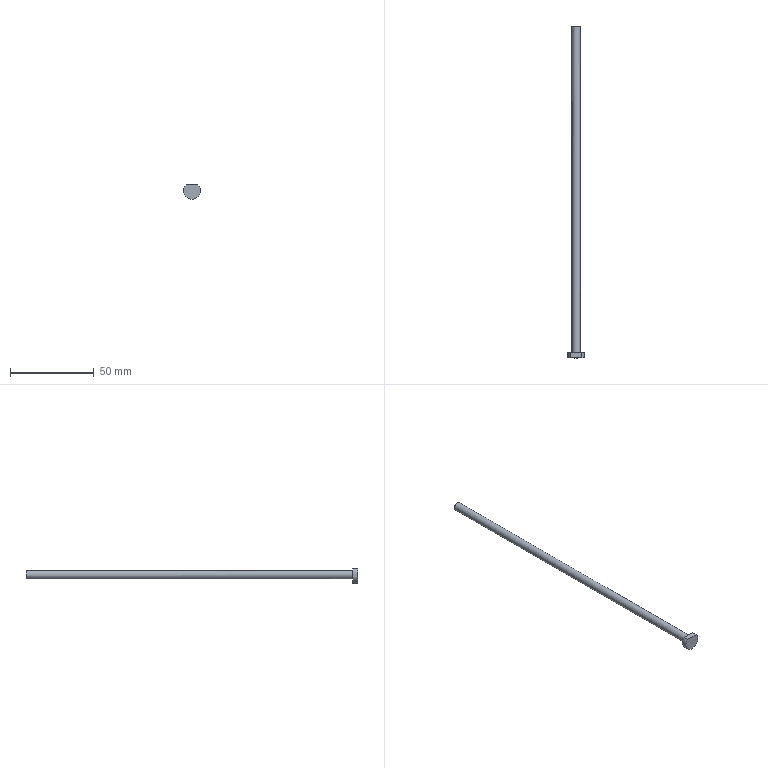Part | STEP file | EJECTION-PIN_id142_x_t | 1 solid | 6 faces | box 10 x 198.09 x 8.5 mm | volume 4042 mm3 | plane 3 | cylinder 3 | commonest cylinder face diameters 5 x1 10 x1 45.097 x1
STEP:
#1=CARTESIAN_POINT('',(-26.429,-220.5,36.73));
#2=VERTEX_POINT('',#1);
#3=CARTESIAN_POINT('',(-33.571,-220.5,36.73));
#4=VERTEX_POINT('',#3);
#5=CARTESIAN_POINT('',(-30.,-220.5,33.23));
#6=DIRECTION('',(0.,1.,0.));
#7=DIRECTION('',(0.,0.,1.));
#8=AXIS2_PLACEMENT_3D('',#5,#6,#7);
#9=CIRCLE('',#8,5.);
#10=EDGE_CURVE('',#2,#4,#9,.T.);
#11=ORIENTED_EDGE('',*,*,#10,.F.);
#12=CARTESIAN_POINT('',(-33.571,-220.5,36.73));
#13=DIRECTION('',(1.,0.,0.));
#14=VECTOR('',#13,1.);
#15=LINE('',#12,#14);
#16=EDGE_CURVE('',#4,#2,#15,.T.);
#17=ORIENTED_EDGE('',*,*,#16,.F.);
#18=EDGE_LOOP('',(#11,#17));
#19=FACE_OUTER_BOUND('',#18,.T.);
#20=CARTESIAN_POINT('',(-30.,-220.5,27.));
#21=DIRECTION('',(0.,1.,0.));
#22=DIRECTION('',(0.,0.,1.));
#23=AXIS2_PLACEMENT_3D('',#20,#21,#22);
#24=PLANE('',#23);
#25=ADVANCED_FACE('',(#19),#24,.F.);
#26=CARTESIAN_POINT('',(-33.571,-217.5,36.73));
#27=VERTEX_POINT('',#26);
#28=CARTESIAN_POINT('',(-33.571,-220.5,36.73));
#29=DIRECTION('',(0.,1.,0.));
#30=VECTOR('',#29,1.);
#31=LINE('',#28,#30);
#32=EDGE_CURVE('',#4,#27,#31,.T.);
#33=ORIENTED_EDGE('',*,*,#32,.F.);
#34=ORIENTED_EDGE('',*,*,#16,.T.);
#35=CARTESIAN_POINT('',(-26.429,-217.5,36.73));
#36=VERTEX_POINT('',#35);
#37=CARTESIAN_POINT('',(-26.429,-220.5,36.73));
#38=DIRECTION('',(0.,-1.,0.));
#39=VECTOR('',#38,1.);
#40=LINE('',#37,#39);
#41=EDGE_CURVE('',#36,#2,#40,.T.);
#42=ORIENTED_EDGE('',*,*,#41,.F.);
#43=CARTESIAN_POINT('',(130.,-217.5,36.73));
#44=DIRECTION('',(1.,0.,0.));
#45=VECTOR('',#44,1.);
#46=LINE('',#43,#45);
#47=EDGE_CURVE('',#27,#36,#46,.T.);
#48=ORIENTED_EDGE('',*,*,#47,.F.);
#49=EDGE_LOOP('',(#33,#34,#42,#48));
#50=FACE_OUTER_BOUND('',#49,.T.);
#51=CARTESIAN_POINT('',(-33.571,-220.5,36.73));
#52=DIRECTION('',(0.,0.,1.));
#53=DIRECTION('',(1.,0.,0.));
#54=AXIS2_PLACEMENT_3D('',#51,#52,#53);
#55=PLANE('',#54);
#56=ADVANCED_FACE('',(#50),#55,.T.);
#57=ORIENTED_EDGE('',*,*,#41,.T.);
#58=ORIENTED_EDGE('',*,*,#10,.T.);
#59=ORIENTED_EDGE('',*,*,#32,.T.);
#60=CARTESIAN_POINT('',(-30.,-217.5,33.23));
#61=DIRECTION('',(0.,1.,0.));
#62=DIRECTION('',(0.,0.,1.));
#63=AXIS2_PLACEMENT_3D('',#60,#61,#62);
#64=CIRCLE('',#63,5.);
#65=EDGE_CURVE('',#36,#27,#64,.T.);
#66=ORIENTED_EDGE('',*,*,#65,.F.);
#67=EDGE_LOOP('',(#57,#58,#59,#66));
#68=FACE_OUTER_BOUND('',#67,.T.);
#69=CARTESIAN_POINT('',(-30.,-220.5,33.23));
#70=DIRECTION('',(0.,1.,0.));
#71=DIRECTION('',(0.,0.,1.));
#72=AXIS2_PLACEMENT_3D('',#69,#70,#71);
#73=CYLINDRICAL_SURFACE('',#72,5.);
#74=ADVANCED_FACE('',(#68),#73,.T.);
#75=CARTESIAN_POINT('',(-27.5,-22.41,33.23));
#76=VERTEX_POINT('',#75);
#77=CARTESIAN_POINT('',(-27.5,-22.41,33.23));
#78=CARTESIAN_POINT('',(-27.5,-22.41,33.509));
#79=CARTESIAN_POINT('',(-27.548,-22.415,33.792));
#80=CARTESIAN_POINT('',(-27.64,-22.425,34.055));
#81=CARTESIAN_POINT('',(-27.732,-22.435,34.318));
#82=CARTESIAN_POINT('',(-27.87,-22.449,34.568));
#83=CARTESIAN_POINT('',(-28.043,-22.464,34.786));
#84=CARTESIAN_POINT('',(-28.217,-22.479,35.005));
#85=CARTESIAN_POINT('',(-28.431,-22.495,35.197));
#86=CARTESIAN_POINT('',(-28.668,-22.509,35.346));
#87=CARTESIAN_POINT('',(-28.905,-22.523,35.495));
#88=CARTESIAN_POINT('',(-29.172,-22.535,35.605));
#89=CARTESIAN_POINT('',(-29.445,-22.542,35.668));
#90=CARTESIAN_POINT('',(-29.717,-22.549,35.73));
#91=CARTESIAN_POINT('',(-30.004,-22.55,35.746));
#92=CARTESIAN_POINT('',(-30.282,-22.547,35.714));
#93=CARTESIAN_POINT('',(-30.559,-22.543,35.683));
#94=CARTESIAN_POINT('',(-30.833,-22.535,35.603));
#95=CARTESIAN_POINT('',(-31.084,-22.523,35.483));
#96=CARTESIAN_POINT('',(-31.335,-22.511,35.362));
#97=CARTESIAN_POINT('',(-31.568,-22.495,35.197));
#98=CARTESIAN_POINT('',(-31.765,-22.479,35.));
#99=CARTESIAN_POINT('',(-31.964,-22.464,34.802));
#100=CARTESIAN_POINT('',(-32.13,-22.448,34.568));
#101=CARTESIAN_POINT('',(-32.252,-22.436,34.316));
#102=CARTESIAN_POINT('',(-32.374,-22.424,34.063));
#103=CARTESIAN_POINT('',(-32.453,-22.415,33.786));
#104=CARTESIAN_POINT('',(-32.485,-22.411,33.508));
#105=CARTESIAN_POINT('',(-32.495,-22.41,33.415));
#106=CARTESIAN_POINT('',(-32.5,-22.41,33.323));
#107=CARTESIAN_POINT('',(-32.5,-22.41,33.23));
#108=CARTESIAN_POINT('',(-32.5,-22.41,32.951));
#109=CARTESIAN_POINT('',(-32.452,-22.415,32.668));
#110=CARTESIAN_POINT('',(-32.36,-22.425,32.405));
#111=CARTESIAN_POINT('',(-32.268,-22.435,32.142));
#112=CARTESIAN_POINT('',(-32.13,-22.449,31.892));
#113=CARTESIAN_POINT('',(-31.957,-22.464,31.674));
#114=CARTESIAN_POINT('',(-31.783,-22.479,31.455));
#115=CARTESIAN_POINT('',(-31.569,-22.495,31.263));
#116=CARTESIAN_POINT('',(-31.332,-22.509,31.114));
#117=CARTESIAN_POINT('',(-31.095,-22.523,30.965));
#118=CARTESIAN_POINT('',(-30.828,-22.535,30.855));
#119=CARTESIAN_POINT('',(-30.555,-22.542,30.792));
#120=CARTESIAN_POINT('',(-30.283,-22.549,30.73));
#121=CARTESIAN_POINT('',(-29.996,-22.55,30.714));
#122=CARTESIAN_POINT('',(-29.718,-22.547,30.746));
#123=CARTESIAN_POINT('',(-29.441,-22.543,30.777));
#124=CARTESIAN_POINT('',(-29.167,-22.535,30.857));
#125=CARTESIAN_POINT('',(-28.916,-22.523,30.977));
#126=CARTESIAN_POINT('',(-28.665,-22.511,31.098));
#127=CARTESIAN_POINT('',(-28.432,-22.495,31.263));
#128=CARTESIAN_POINT('',(-28.235,-22.479,31.46));
#129=CARTESIAN_POINT('',(-28.036,-22.464,31.658));
#130=CARTESIAN_POINT('',(-27.87,-22.448,31.892));
#131=CARTESIAN_POINT('',(-27.748,-22.436,32.144));
#132=CARTESIAN_POINT('',(-27.626,-22.424,32.397));
#133=CARTESIAN_POINT('',(-27.547,-22.415,32.674));
#134=CARTESIAN_POINT('',(-27.515,-22.411,32.952));
#135=CARTESIAN_POINT('',(-27.505,-22.41,33.045));
#136=CARTESIAN_POINT('',(-27.5,-22.41,33.137));
#137=CARTESIAN_POINT('',(-27.5,-22.41,33.23));
#138=B_SPLINE_CURVE_WITH_KNOTS('',3,(#77,#78,#79,#80,#81,#82,#83,#84,#85,#86,#87,#88,#89,#90,#91,#92,#93,#94,#95,#96,#97,#98,#99,#100,#101,#102,#103,#104,#105,#106,#107,#108,#109,#110,#111,#112,#113,#114,#115,#116,#117,#118,#119,#120,#121,#122,#123,#124,#125,#126,#127,#128,#129,#130,#131,#132,#133,#134,#135,#136,#137),.UNSPECIFIED.,.T.,.F.,(1,3,3,3,3,3,3,3,3,3,3,3,3,3,3,3,3,3,3,3,3,3,1),(-0.01755,0.,0.05349,0.107,0.1606,0.2145,0.2681,0.3214,0.3749,0.4287,0.4825,0.5,0.5535,0.607,0.6606,0.7145,0.7681,0.8214,0.8749,0.9287,0.9825,1.,1.053),.UNSPECIFIED.);
#139=EDGE_CURVE('',#76,#76,#138,.T.);
#140=ORIENTED_EDGE('',*,*,#139,.F.);
#141=EDGE_LOOP('',(#140));
#142=FACE_OUTER_BOUND('',#141,.T.);
#143=CARTESIAN_POINT('',(-30.,0.,41.761));
#144=DIRECTION('',(0.,0.,1.));
#145=DIRECTION('',(1.,0.,0.));
#146=AXIS2_PLACEMENT_3D('',#143,#144,#145);
#147=CYLINDRICAL_SURFACE('',#146,22.549);
#148=ADVANCED_FACE('',(#142),#147,.F.);
#149=CARTESIAN_POINT('',(-30.,-217.5,35.73));
#150=VERTEX_POINT('',#149);
#151=CARTESIAN_POINT('',(-30.,-217.5,33.23));
#152=DIRECTION('',(0.,1.,0.));
#153=DIRECTION('',(0.,0.,1.));
#154=AXIS2_PLACEMENT_3D('',#151,#152,#153);
#155=CIRCLE('',#154,2.5);
#156=EDGE_CURVE('',#150,#150,#155,.T.);
#157=ORIENTED_EDGE('',*,*,#156,.F.);
#158=EDGE_LOOP('',(#157));
#159=FACE_BOUND('',#158,.T.);
#160=ORIENTED_EDGE('',*,*,#47,.T.);
#161=ORIENTED_EDGE('',*,*,#65,.T.);
#162=EDGE_LOOP('',(#160,#161));
#163=FACE_BOUND('',#162,.T.);
#164=CARTESIAN_POINT('',(130.,-217.5,-52.5));
#165=DIRECTION('',(0.,1.,0.));
#166=DIRECTION('',(0.,0.,1.));
#167=AXIS2_PLACEMENT_3D('',#164,#165,#166);
#168=PLANE('',#167);
#169=ADVANCED_FACE('',(#159,#163),#168,.T.);
#170=ORIENTED_EDGE('',*,*,#139,.T.);
#171=EDGE_LOOP('',(#170));
#172=FACE_BOUND('',#171,.T.);
#173=ORIENTED_EDGE('',*,*,#156,.T.);
#174=EDGE_LOOP('',(#173));
#175=FACE_BOUND('',#174,.T.);
#176=CARTESIAN_POINT('',(-30.,0.,33.23));
#177=DIRECTION('',(0.,1.,0.));
#178=DIRECTION('',(0.,0.,1.));
#179=AXIS2_PLACEMENT_3D('',#176,#177,#178);
#180=CYLINDRICAL_SURFACE('',#179,2.5);
#181=ADVANCED_FACE('',(#172,#175),#180,.T.);
#182=CLOSED_SHELL('',(#25,#56,#74,#148,#169,#181));
#183=MANIFOLD_SOLID_BREP('',#182);
#184=(LENGTH_UNIT()NAMED_UNIT(*)SI_UNIT(.MILLI.,.METRE.));
#185=UNCERTAINTY_MEASURE_WITH_UNIT(LENGTH_MEASURE(0.0508),#184,'','');
#186=(NAMED_UNIT(*)PLANE_ANGLE_UNIT()SI_UNIT($,.RADIAN.));
#187=PLANE_ANGLE_MEASURE_WITH_UNIT(PLANE_ANGLE_MEASURE(0.01745),#186);
#188=DIMENSIONAL_EXPONENTS(0.,0.,0.,0.,0.,0.,0.);
#189=(CONVERSION_BASED_UNIT('DEGREE',#187)NAMED_UNIT(#188)PLANE_ANGLE_UNIT());
#190=(NAMED_UNIT(*)SI_UNIT($,.STERADIAN.)SOLID_ANGLE_UNIT());
#191=(GEOMETRIC_REPRESENTATION_CONTEXT(3)GLOBAL_UNCERTAINTY_ASSIGNED_CONTEXT((#185))GLOBAL_UNIT_ASSIGNED_CONTEXT((#184,#189,#190))REPRESENTATION_CONTEXT('',''));
#192=ADVANCED_BREP_SHAPE_REPRESENTATION('',(#183),#191);